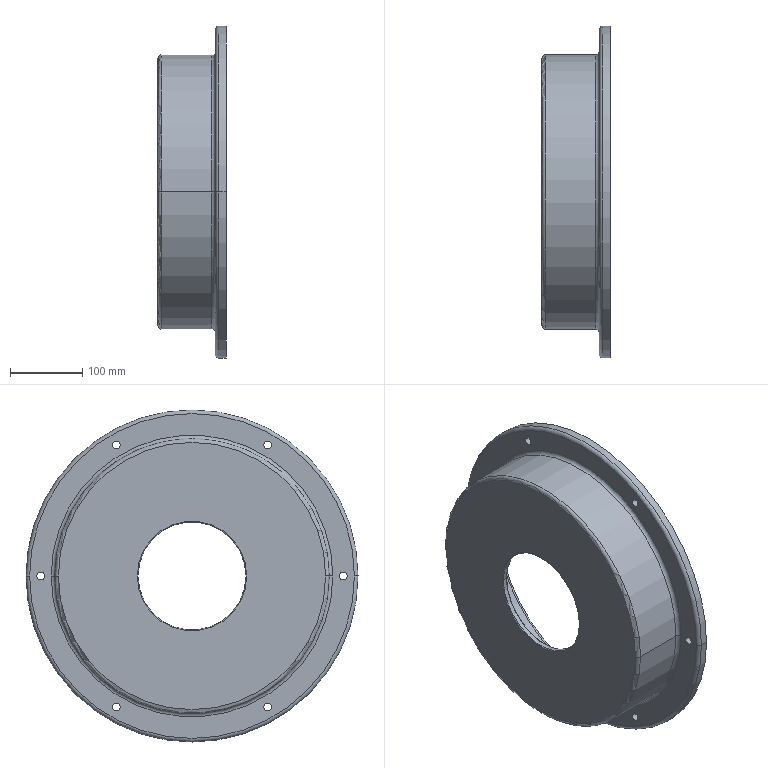Part | SolidWorks | features Cut 1, Revolution 1 | 1 solid | 43 faces | box 94.6 x 461 x 461 mm | volume 3440559 mm3 | cylinder 22 | torus 16 | plane 5 | commonest cylinder face diameters 11 x12 150 x2 225 x2 351 x2 381 x2 461 x2
STEP:
#1=CARTESIAN_POINT('',(298.52,204.5,0.));
#2=VERTEX_POINT('',#1);
#3=CARTESIAN_POINT('',(298.52,215.5,0.));
#4=VERTEX_POINT('',#3);
#5=CARTESIAN_POINT('',(298.52,210.,0.));
#6=DIRECTION('',(1.,0.,0.));
#7=DIRECTION('',(0.,1.,0.));
#8=AXIS2_PLACEMENT_3D('',#5,#6,#7);
#9=CIRCLE('',#8,5.5);
#10=EDGE_CURVE('',#2,#4,#9,.T.);
#11=ORIENTED_EDGE('',*,*,#10,.T.);
#12=CARTESIAN_POINT('',(283.52,215.5,0.));
#13=VERTEX_POINT('',#12);
#14=CARTESIAN_POINT('',(368.52,215.5,0.));
#15=DIRECTION('',(-1.,0.,0.));
#16=VECTOR('',#15,1000.);
#17=LINE('',#14,#16);
#18=EDGE_CURVE('',#4,#13,#17,.T.);
#19=ORIENTED_EDGE('',*,*,#18,.T.);
#20=CARTESIAN_POINT('',(283.52,204.5,0.));
#21=VERTEX_POINT('',#20);
#22=CARTESIAN_POINT('',(283.52,210.,0.));
#23=DIRECTION('',(-1.,0.,0.));
#24=DIRECTION('',(0.,-1.,0.));
#25=AXIS2_PLACEMENT_3D('',#22,#23,#24);
#26=CIRCLE('',#25,5.5);
#27=EDGE_CURVE('',#13,#21,#26,.T.);
#28=ORIENTED_EDGE('',*,*,#27,.T.);
#29=CARTESIAN_POINT('',(368.52,204.5,0.));
#30=DIRECTION('',(-1.,0.,0.));
#31=VECTOR('',#30,1000.);
#32=LINE('',#29,#31);
#33=EDGE_CURVE('',#2,#21,#32,.T.);
#34=ORIENTED_EDGE('',*,*,#33,.F.);
#35=EDGE_LOOP('',(#11,#19,#28,#34));
#36=FACE_OUTER_BOUND('',#35,.T.);
#37=CARTESIAN_POINT('',(368.52,210.,0.));
#38=DIRECTION('',(-1.,0.,0.));
#39=DIRECTION('',(0.,-1.,0.));
#40=AXIS2_PLACEMENT_3D('',#37,#38,#39);
#41=CYLINDRICAL_SURFACE('',#40,5.5);
#42=ADVANCED_FACE('',(#36),#41,.F.);
#43=CARTESIAN_POINT('',(298.52,99.5,-181.865));
#44=VERTEX_POINT('',#43);
#45=CARTESIAN_POINT('',(298.52,110.5,-181.865));
#46=VERTEX_POINT('',#45);
#47=CARTESIAN_POINT('',(298.52,105.,-181.865));
#48=DIRECTION('',(1.,0.,0.));
#49=DIRECTION('',(0.,1.,0.));
#50=AXIS2_PLACEMENT_3D('',#47,#48,#49);
#51=CIRCLE('',#50,5.5);
#52=EDGE_CURVE('',#44,#46,#51,.T.);
#53=ORIENTED_EDGE('',*,*,#52,.T.);
#54=CARTESIAN_POINT('',(283.52,110.5,-181.865));
#55=VERTEX_POINT('',#54);
#56=CARTESIAN_POINT('',(368.52,110.5,-181.865));
#57=DIRECTION('',(-1.,0.,0.));
#58=VECTOR('',#57,1000.);
#59=LINE('',#56,#58);
#60=EDGE_CURVE('',#46,#55,#59,.T.);
#61=ORIENTED_EDGE('',*,*,#60,.T.);
#62=CARTESIAN_POINT('',(283.52,99.5,-181.865));
#63=VERTEX_POINT('',#62);
#64=CARTESIAN_POINT('',(283.52,105.,-181.865));
#65=DIRECTION('',(-1.,0.,0.));
#66=DIRECTION('',(0.,-1.,0.));
#67=AXIS2_PLACEMENT_3D('',#64,#65,#66);
#68=CIRCLE('',#67,5.5);
#69=EDGE_CURVE('',#55,#63,#68,.T.);
#70=ORIENTED_EDGE('',*,*,#69,.T.);
#71=CARTESIAN_POINT('',(368.52,99.5,-181.865));
#72=DIRECTION('',(-1.,0.,0.));
#73=VECTOR('',#72,1000.);
#74=LINE('',#71,#73);
#75=EDGE_CURVE('',#44,#63,#74,.T.);
#76=ORIENTED_EDGE('',*,*,#75,.F.);
#77=EDGE_LOOP('',(#53,#61,#70,#76));
#78=FACE_OUTER_BOUND('',#77,.T.);
#79=CARTESIAN_POINT('',(368.52,105.,-181.865));
#80=DIRECTION('',(-1.,0.,0.));
#81=DIRECTION('',(0.,-1.,0.));
#82=AXIS2_PLACEMENT_3D('',#79,#80,#81);
#83=CYLINDRICAL_SURFACE('',#82,5.5);
#84=ADVANCED_FACE('',(#78),#83,.F.);
#85=CARTESIAN_POINT('',(298.52,-110.5,-181.865));
#86=VERTEX_POINT('',#85);
#87=CARTESIAN_POINT('',(298.52,-99.5,-181.865));
#88=VERTEX_POINT('',#87);
#89=CARTESIAN_POINT('',(298.52,-105.,-181.865));
#90=DIRECTION('',(1.,0.,0.));
#91=DIRECTION('',(0.,1.,0.));
#92=AXIS2_PLACEMENT_3D('',#89,#90,#91);
#93=CIRCLE('',#92,5.5);
#94=EDGE_CURVE('',#86,#88,#93,.T.);
#95=ORIENTED_EDGE('',*,*,#94,.T.);
#96=CARTESIAN_POINT('',(283.52,-99.5,-181.865));
#97=VERTEX_POINT('',#96);
#98=CARTESIAN_POINT('',(368.52,-99.5,-181.865));
#99=DIRECTION('',(-1.,0.,0.));
#100=VECTOR('',#99,1000.);
#101=LINE('',#98,#100);
#102=EDGE_CURVE('',#88,#97,#101,.T.);
#103=ORIENTED_EDGE('',*,*,#102,.T.);
#104=CARTESIAN_POINT('',(283.52,-110.5,-181.865));
#105=VERTEX_POINT('',#104);
#106=CARTESIAN_POINT('',(283.52,-105.,-181.865));
#107=DIRECTION('',(-1.,0.,0.));
#108=DIRECTION('',(0.,-1.,0.));
#109=AXIS2_PLACEMENT_3D('',#106,#107,#108);
#110=CIRCLE('',#109,5.5);
#111=EDGE_CURVE('',#97,#105,#110,.T.);
#112=ORIENTED_EDGE('',*,*,#111,.T.);
#113=CARTESIAN_POINT('',(368.52,-110.5,-181.865));
#114=DIRECTION('',(-1.,0.,0.));
#115=VECTOR('',#114,1000.);
#116=LINE('',#113,#115);
#117=EDGE_CURVE('',#86,#105,#116,.T.);
#118=ORIENTED_EDGE('',*,*,#117,.F.);
#119=EDGE_LOOP('',(#95,#103,#112,#118));
#120=FACE_OUTER_BOUND('',#119,.T.);
#121=CARTESIAN_POINT('',(368.52,-105.,-181.865));
#122=DIRECTION('',(-1.,0.,0.));
#123=DIRECTION('',(0.,-1.,0.));
#124=AXIS2_PLACEMENT_3D('',#121,#122,#123);
#125=CYLINDRICAL_SURFACE('',#124,5.5);
#126=ADVANCED_FACE('',(#120),#125,.F.);
#127=CARTESIAN_POINT('',(298.52,-215.5,0.));
#128=VERTEX_POINT('',#127);
#129=CARTESIAN_POINT('',(298.52,-204.5,0.));
#130=VERTEX_POINT('',#129);
#131=CARTESIAN_POINT('',(298.52,-210.,0.));
#132=DIRECTION('',(1.,0.,0.));
#133=DIRECTION('',(0.,1.,0.));
#134=AXIS2_PLACEMENT_3D('',#131,#132,#133);
#135=CIRCLE('',#134,5.5);
#136=EDGE_CURVE('',#128,#130,#135,.T.);
#137=ORIENTED_EDGE('',*,*,#136,.T.);
#138=CARTESIAN_POINT('',(283.52,-204.5,0.));
#139=VERTEX_POINT('',#138);
#140=CARTESIAN_POINT('',(368.52,-204.5,0.));
#141=DIRECTION('',(-1.,0.,0.));
#142=VECTOR('',#141,1000.);
#143=LINE('',#140,#142);
#144=EDGE_CURVE('',#130,#139,#143,.T.);
#145=ORIENTED_EDGE('',*,*,#144,.T.);
#146=CARTESIAN_POINT('',(283.52,-215.5,0.));
#147=VERTEX_POINT('',#146);
#148=CARTESIAN_POINT('',(283.52,-210.,0.));
#149=DIRECTION('',(-1.,0.,0.));
#150=DIRECTION('',(0.,-1.,0.));
#151=AXIS2_PLACEMENT_3D('',#148,#149,#150);
#152=CIRCLE('',#151,5.5);
#153=EDGE_CURVE('',#139,#147,#152,.T.);
#154=ORIENTED_EDGE('',*,*,#153,.T.);
#155=CARTESIAN_POINT('',(368.52,-215.5,0.));
#156=DIRECTION('',(-1.,0.,0.));
#157=VECTOR('',#156,1000.);
#158=LINE('',#155,#157);
#159=EDGE_CURVE('',#128,#147,#158,.T.);
#160=ORIENTED_EDGE('',*,*,#159,.F.);
#161=EDGE_LOOP('',(#137,#145,#154,#160));
#162=FACE_OUTER_BOUND('',#161,.T.);
#163=CARTESIAN_POINT('',(368.52,-210.,0.));
#164=DIRECTION('',(-1.,0.,0.));
#165=DIRECTION('',(0.,-1.,0.));
#166=AXIS2_PLACEMENT_3D('',#163,#164,#165);
#167=CYLINDRICAL_SURFACE('',#166,5.5);
#168=ADVANCED_FACE('',(#162),#167,.F.);
#169=CARTESIAN_POINT('',(298.52,-110.5,181.865));
#170=VERTEX_POINT('',#169);
#171=CARTESIAN_POINT('',(298.52,-99.5,181.865));
#172=VERTEX_POINT('',#171);
#173=CARTESIAN_POINT('',(298.52,-105.,181.865));
#174=DIRECTION('',(1.,0.,0.));
#175=DIRECTION('',(0.,1.,0.));
#176=AXIS2_PLACEMENT_3D('',#173,#174,#175);
#177=CIRCLE('',#176,5.5);
#178=EDGE_CURVE('',#170,#172,#177,.T.);
#179=ORIENTED_EDGE('',*,*,#178,.T.);
#180=CARTESIAN_POINT('',(283.52,-99.5,181.865));
#181=VERTEX_POINT('',#180);
#182=CARTESIAN_POINT('',(368.52,-99.5,181.865));
#183=DIRECTION('',(-1.,0.,0.));
#184=VECTOR('',#183,1000.);
#185=LINE('',#182,#184);
#186=EDGE_CURVE('',#172,#181,#185,.T.);
#187=ORIENTED_EDGE('',*,*,#186,.T.);
#188=CARTESIAN_POINT('',(283.52,-110.5,181.865));
#189=VERTEX_POINT('',#188);
#190=CARTESIAN_POINT('',(283.52,-105.,181.865));
#191=DIRECTION('',(-1.,0.,0.));
#192=DIRECTION('',(0.,-1.,0.));
#193=AXIS2_PLACEMENT_3D('',#190,#191,#192);
#194=CIRCLE('',#193,5.5);
#195=EDGE_CURVE('',#181,#189,#194,.T.);
#196=ORIENTED_EDGE('',*,*,#195,.T.);
#197=CARTESIAN_POINT('',(368.52,-110.5,181.865));
#198=DIRECTION('',(-1.,0.,0.));
#199=VECTOR('',#198,1000.);
#200=LINE('',#197,#199);
#201=EDGE_CURVE('',#170,#189,#200,.T.);
#202=ORIENTED_EDGE('',*,*,#201,.F.);
#203=EDGE_LOOP('',(#179,#187,#196,#202));
#204=FACE_OUTER_BOUND('',#203,.T.);
#205=CARTESIAN_POINT('',(368.52,-105.,181.865));
#206=DIRECTION('',(-1.,0.,0.));
#207=DIRECTION('',(0.,-1.,0.));
#208=AXIS2_PLACEMENT_3D('',#205,#206,#207);
#209=CYLINDRICAL_SURFACE('',#208,5.5);
#210=ADVANCED_FACE('',(#204),#209,.F.);
#211=CARTESIAN_POINT('',(298.52,99.5,181.865));
#212=VERTEX_POINT('',#211);
#213=CARTESIAN_POINT('',(298.52,110.5,181.865));
#214=VERTEX_POINT('',#213);
#215=CARTESIAN_POINT('',(298.52,105.,181.865));
#216=DIRECTION('',(1.,0.,0.));
#217=DIRECTION('',(0.,1.,0.));
#218=AXIS2_PLACEMENT_3D('',#215,#216,#217);
#219=CIRCLE('',#218,5.5);
#220=EDGE_CURVE('',#212,#214,#219,.T.);
#221=ORIENTED_EDGE('',*,*,#220,.T.);
#222=CARTESIAN_POINT('',(283.52,110.5,181.865));
#223=VERTEX_POINT('',#222);
#224=CARTESIAN_POINT('',(368.52,110.5,181.865));
#225=DIRECTION('',(-1.,0.,0.));
#226=VECTOR('',#225,1000.);
#227=LINE('',#224,#226);
#228=EDGE_CURVE('',#214,#223,#227,.T.);
#229=ORIENTED_EDGE('',*,*,#228,.T.);
#230=CARTESIAN_POINT('',(283.52,99.5,181.865));
#231=VERTEX_POINT('',#230);
#232=CARTESIAN_POINT('',(283.52,105.,181.865));
#233=DIRECTION('',(-1.,0.,0.));
#234=DIRECTION('',(0.,-1.,0.));
#235=AXIS2_PLACEMENT_3D('',#232,#233,#234);
#236=CIRCLE('',#235,5.5);
#237=EDGE_CURVE('',#223,#231,#236,.T.);
#238=ORIENTED_EDGE('',*,*,#237,.T.);
#239=CARTESIAN_POINT('',(368.52,99.5,181.865));
#240=DIRECTION('',(-1.,0.,0.));
#241=VECTOR('',#240,1000.);
#242=LINE('',#239,#241);
#243=EDGE_CURVE('',#212,#231,#242,.T.);
#244=ORIENTED_EDGE('',*,*,#243,.F.);
#245=EDGE_LOOP('',(#221,#229,#238,#244));
#246=FACE_OUTER_BOUND('',#245,.T.);
#247=CARTESIAN_POINT('',(368.52,105.,181.865));
#248=DIRECTION('',(-1.,0.,0.));
#249=DIRECTION('',(0.,-1.,0.));
#250=AXIS2_PLACEMENT_3D('',#247,#248,#249);
#251=CYLINDRICAL_SURFACE('',#250,5.5);
#252=ADVANCED_FACE('',(#246),#251,.F.);
#253=CARTESIAN_POINT('',(212.92,-112.5,0.));
#254=VERTEX_POINT('',#253);
#255=CARTESIAN_POINT('',(212.92,112.5,0.));
#256=VERTEX_POINT('',#255);
#257=CARTESIAN_POINT('',(212.92,0.,0.));
#258=DIRECTION('',(1.,0.,0.));
#259=DIRECTION('',(0.,1.,0.));
#260=AXIS2_PLACEMENT_3D('',#257,#258,#259);
#261=CIRCLE('',#260,112.5);
#262=EDGE_CURVE('',#254,#256,#261,.T.);
#263=ORIENTED_EDGE('',*,*,#262,.F.);
#264=CARTESIAN_POINT('',(218.92,-112.5,0.));
#265=VERTEX_POINT('',#264);
#266=CARTESIAN_POINT('',(373.52,-112.5,0.));
#267=DIRECTION('',(1.,0.,0.));
#268=VECTOR('',#267,1000.);
#269=LINE('',#266,#268);
#270=EDGE_CURVE('',#254,#265,#269,.T.);
#271=ORIENTED_EDGE('',*,*,#270,.T.);
#272=CARTESIAN_POINT('',(218.92,112.5,0.));
#273=VERTEX_POINT('',#272);
#274=CARTESIAN_POINT('',(218.92,0.,0.));
#275=DIRECTION('',(1.,0.,0.));
#276=DIRECTION('',(0.,1.,0.));
#277=AXIS2_PLACEMENT_3D('',#274,#275,#276);
#278=CIRCLE('',#277,112.5);
#279=EDGE_CURVE('',#265,#273,#278,.T.);
#280=ORIENTED_EDGE('',*,*,#279,.T.);
#281=CARTESIAN_POINT('',(373.52,112.5,0.));
#282=DIRECTION('',(1.,0.,0.));
#283=VECTOR('',#282,1000.);
#284=LINE('',#281,#283);
#285=EDGE_CURVE('',#256,#273,#284,.T.);
#286=ORIENTED_EDGE('',*,*,#285,.F.);
#287=EDGE_LOOP('',(#263,#271,#280,#286));
#288=FACE_OUTER_BOUND('',#287,.T.);
#289=CARTESIAN_POINT('',(373.52,0.,0.));
#290=DIRECTION('',(1.,0.,0.));
#291=DIRECTION('',(0.,1.,0.));
#292=AXIS2_PLACEMENT_3D('',#289,#290,#291);
#293=CYLINDRICAL_SURFACE('',#292,112.5);
#294=ADVANCED_FACE('',(#288),#293,.F.);
#295=CARTESIAN_POINT('',(211.92,-111.5,0.));
#296=VERTEX_POINT('',#295);
#297=CARTESIAN_POINT('',(211.92,111.5,0.));
#298=VERTEX_POINT('',#297);
#299=CARTESIAN_POINT('',(211.92,0.,0.));
#300=DIRECTION('',(1.,0.,0.));
#301=DIRECTION('',(0.,1.,0.));
#302=AXIS2_PLACEMENT_3D('',#299,#300,#301);
#303=CIRCLE('',#302,111.5);
#304=EDGE_CURVE('',#296,#298,#303,.T.);
#305=ORIENTED_EDGE('',*,*,#304,.F.);
#306=CARTESIAN_POINT('',(212.92,-111.5,0.));
#307=DIRECTION('',(0.,0.,1.));
#308=DIRECTION('',(0.,-1.,0.));
#309=AXIS2_PLACEMENT_3D('',#306,#307,#308);
#310=CIRCLE('',#309,1.);
#311=EDGE_CURVE('',#296,#254,#310,.T.);
#312=ORIENTED_EDGE('',*,*,#311,.T.);
#313=ORIENTED_EDGE('',*,*,#262,.T.);
#314=CARTESIAN_POINT('',(212.92,111.5,0.));
#315=DIRECTION('',(0.,0.,-1.));
#316=DIRECTION('',(-1.,0.,0.));
#317=AXIS2_PLACEMENT_3D('',#314,#315,#316);
#318=CIRCLE('',#317,1.);
#319=EDGE_CURVE('',#298,#256,#318,.T.);
#320=ORIENTED_EDGE('',*,*,#319,.F.);
#321=EDGE_LOOP('',(#305,#312,#313,#320));
#322=FACE_OUTER_BOUND('',#321,.T.);
#323=CARTESIAN_POINT('',(212.92,0.,0.));
#324=DIRECTION('',(1.,0.,0.));
#325=DIRECTION('',(0.,1.,0.));
#326=AXIS2_PLACEMENT_3D('',#323,#324,#325);
#327=TOROIDAL_SURFACE('',#326,111.5,1.);
#328=ADVANCED_FACE('',(#322),#327,.F.);
#329=CARTESIAN_POINT('',(211.92,76.,0.));
#330=VERTEX_POINT('',#329);
#331=CARTESIAN_POINT('',(211.92,-76.,0.));
#332=VERTEX_POINT('',#331);
#333=CARTESIAN_POINT('',(211.92,0.,0.));
#334=DIRECTION('',(1.,0.,0.));
#335=DIRECTION('',(0.,1.,0.));
#336=AXIS2_PLACEMENT_3D('',#333,#334,#335);
#337=CIRCLE('',#336,76.);
#338=EDGE_CURVE('',#330,#332,#337,.T.);
#339=ORIENTED_EDGE('',*,*,#338,.T.);
#340=CARTESIAN_POINT('',(210.92,-75.,0.));
#341=VERTEX_POINT('',#340);
#342=CARTESIAN_POINT('',(210.92,-76.,0.));
#343=DIRECTION('',(0.,0.,1.));
#344=DIRECTION('',(0.,-1.,0.));
#345=AXIS2_PLACEMENT_3D('',#342,#343,#344);
#346=CIRCLE('',#345,1.);
#347=EDGE_CURVE('',#332,#341,#346,.T.);
#348=ORIENTED_EDGE('',*,*,#347,.T.);
#349=CARTESIAN_POINT('',(210.92,75.,0.));
#350=VERTEX_POINT('',#349);
#351=CARTESIAN_POINT('',(210.92,0.,0.));
#352=DIRECTION('',(1.,0.,0.));
#353=DIRECTION('',(0.,1.,0.));
#354=AXIS2_PLACEMENT_3D('',#351,#352,#353);
#355=CIRCLE('',#354,75.);
#356=EDGE_CURVE('',#350,#341,#355,.T.);
#357=ORIENTED_EDGE('',*,*,#356,.F.);
#358=CARTESIAN_POINT('',(210.92,76.,0.));
#359=DIRECTION('',(0.,0.,-1.));
#360=DIRECTION('',(-1.,0.,0.));
#361=AXIS2_PLACEMENT_3D('',#358,#359,#360);
#362=CIRCLE('',#361,1.);
#363=EDGE_CURVE('',#330,#350,#362,.T.);
#364=ORIENTED_EDGE('',*,*,#363,.F.);
#365=EDGE_LOOP('',(#339,#348,#357,#364));
#366=FACE_OUTER_BOUND('',#365,.T.);
#367=CARTESIAN_POINT('',(210.92,0.,0.));
#368=DIRECTION('',(1.,0.,0.));
#369=DIRECTION('',(0.,1.,0.));
#370=AXIS2_PLACEMENT_3D('',#367,#368,#369);
#371=TOROIDAL_SURFACE('',#370,76.,1.);
#372=ADVANCED_FACE('',(#366),#371,.T.);
#373=CARTESIAN_POINT('',(204.92,-75.,0.));
#374=VERTEX_POINT('',#373);
#375=CARTESIAN_POINT('',(204.92,75.,0.));
#376=VERTEX_POINT('',#375);
#377=CARTESIAN_POINT('',(204.92,0.,0.));
#378=DIRECTION('',(1.,0.,0.));
#379=DIRECTION('',(0.,1.,0.));
#380=AXIS2_PLACEMENT_3D('',#377,#378,#379);
#381=CIRCLE('',#380,75.);
#382=EDGE_CURVE('',#374,#376,#381,.T.);
#383=ORIENTED_EDGE('',*,*,#382,.F.);
#384=CARTESIAN_POINT('',(373.52,-75.,0.));
#385=DIRECTION('',(1.,0.,0.));
#386=VECTOR('',#385,1000.);
#387=LINE('',#384,#386);
#388=EDGE_CURVE('',#374,#341,#387,.T.);
#389=ORIENTED_EDGE('',*,*,#388,.T.);
#390=CARTESIAN_POINT('',(210.92,0.,0.));
#391=DIRECTION('',(1.,0.,0.));
#392=DIRECTION('',(0.,1.,0.));
#393=AXIS2_PLACEMENT_3D('',#390,#391,#392);
#394=CIRCLE('',#393,75.);
#395=EDGE_CURVE('',#341,#350,#394,.T.);
#396=ORIENTED_EDGE('',*,*,#395,.T.);
#397=CARTESIAN_POINT('',(373.52,75.,0.));
#398=DIRECTION('',(1.,0.,0.));
#399=VECTOR('',#398,1000.);
#400=LINE('',#397,#399);
#401=EDGE_CURVE('',#376,#350,#400,.T.);
#402=ORIENTED_EDGE('',*,*,#401,.F.);
#403=EDGE_LOOP('',(#383,#389,#396,#402));
#404=FACE_OUTER_BOUND('',#403,.T.);
#405=CARTESIAN_POINT('',(373.52,0.,0.));
#406=DIRECTION('',(1.,0.,0.));
#407=DIRECTION('',(0.,1.,0.));
#408=AXIS2_PLACEMENT_3D('',#405,#406,#407);
#409=CYLINDRICAL_SURFACE('',#408,75.);
#410=ADVANCED_FACE('',(#404),#409,.F.);
#411=CARTESIAN_POINT('',(204.92,0.,0.));
#412=DIRECTION('',(1.,0.,0.));
#413=DIRECTION('',(0.,1.,0.));
#414=AXIS2_PLACEMENT_3D('',#411,#412,#413);
#415=CIRCLE('',#414,75.);
#416=EDGE_CURVE('',#376,#374,#415,.T.);
#417=ORIENTED_EDGE('',*,*,#416,.T.);
#418=CARTESIAN_POINT('',(203.92,-76.,0.));
#419=VERTEX_POINT('',#418);
#420=CARTESIAN_POINT('',(204.92,-76.,0.));
#421=DIRECTION('',(0.,0.,1.));
#422=DIRECTION('',(0.,-1.,0.));
#423=AXIS2_PLACEMENT_3D('',#420,#421,#422);
#424=CIRCLE('',#423,1.);
#425=EDGE_CURVE('',#374,#419,#424,.T.);
#426=ORIENTED_EDGE('',*,*,#425,.T.);
#427=CARTESIAN_POINT('',(203.92,76.,0.));
#428=VERTEX_POINT('',#427);
#429=CARTESIAN_POINT('',(203.92,0.,0.));
#430=DIRECTION('',(1.,0.,0.));
#431=DIRECTION('',(0.,1.,0.));
#432=AXIS2_PLACEMENT_3D('',#429,#430,#431);
#433=CIRCLE('',#432,76.);
#434=EDGE_CURVE('',#428,#419,#433,.T.);
#435=ORIENTED_EDGE('',*,*,#434,.F.);
#436=CARTESIAN_POINT('',(204.92,76.,0.));
#437=DIRECTION('',(0.,0.,-1.));
#438=DIRECTION('',(-1.,0.,0.));
#439=AXIS2_PLACEMENT_3D('',#436,#437,#438);
#440=CIRCLE('',#439,1.);
#441=EDGE_CURVE('',#376,#428,#440,.T.);
#442=ORIENTED_EDGE('',*,*,#441,.F.);
#443=EDGE_LOOP('',(#417,#426,#435,#442));
#444=FACE_OUTER_BOUND('',#443,.T.);
#445=CARTESIAN_POINT('',(204.92,0.,0.));
#446=DIRECTION('',(1.,0.,0.));
#447=DIRECTION('',(0.,1.,0.));
#448=AXIS2_PLACEMENT_3D('',#445,#446,#447);
#449=TOROIDAL_SURFACE('',#448,76.,1.);
#450=ADVANCED_FACE('',(#444),#449,.T.);
#451=CARTESIAN_POINT('',(203.92,185.5,0.));
#452=VERTEX_POINT('',#451);
#453=CARTESIAN_POINT('',(203.92,-185.5,0.));
#454=VERTEX_POINT('',#453);
#455=CARTESIAN_POINT('',(203.92,0.,0.));
#456=DIRECTION('',(1.,0.,0.));
#457=DIRECTION('',(0.,1.,0.));
#458=AXIS2_PLACEMENT_3D('',#455,#456,#457);
#459=CIRCLE('',#458,185.5);
#460=EDGE_CURVE('',#452,#454,#459,.T.);
#461=ORIENTED_EDGE('',*,*,#460,.T.);
#462=CARTESIAN_POINT('',(208.92,-190.5,0.));
#463=VERTEX_POINT('',#462);
#464=CARTESIAN_POINT('',(208.92,-185.5,0.));
#465=DIRECTION('',(0.,0.,1.));
#466=DIRECTION('',(0.,-1.,0.));
#467=AXIS2_PLACEMENT_3D('',#464,#465,#466);
#468=CIRCLE('',#467,5.);
#469=EDGE_CURVE('',#454,#463,#468,.T.);
#470=ORIENTED_EDGE('',*,*,#469,.T.);
#471=CARTESIAN_POINT('',(208.92,190.5,0.));
#472=VERTEX_POINT('',#471);
#473=CARTESIAN_POINT('',(208.92,0.,0.));
#474=DIRECTION('',(1.,0.,0.));
#475=DIRECTION('',(0.,1.,0.));
#476=AXIS2_PLACEMENT_3D('',#473,#474,#475);
#477=CIRCLE('',#476,190.5);
#478=EDGE_CURVE('',#472,#463,#477,.T.);
#479=ORIENTED_EDGE('',*,*,#478,.F.);
#480=CARTESIAN_POINT('',(208.92,185.5,0.));
#481=DIRECTION('',(0.,0.,-1.));
#482=DIRECTION('',(-1.,0.,0.));
#483=AXIS2_PLACEMENT_3D('',#480,#481,#482);
#484=CIRCLE('',#483,5.);
#485=EDGE_CURVE('',#452,#472,#484,.T.);
#486=ORIENTED_EDGE('',*,*,#485,.F.);
#487=EDGE_LOOP('',(#461,#470,#479,#486));
#488=FACE_OUTER_BOUND('',#487,.T.);
#489=CARTESIAN_POINT('',(208.92,0.,0.));
#490=DIRECTION('',(1.,0.,0.));
#491=DIRECTION('',(0.,1.,0.));
#492=AXIS2_PLACEMENT_3D('',#489,#490,#491);
#493=TOROIDAL_SURFACE('',#492,185.5,5.);
#494=ADVANCED_FACE('',(#488),#493,.T.);
#495=ORIENTED_EDGE('',*,*,#478,.T.);
#496=CARTESIAN_POINT('',(278.52,-190.5,0.));
#497=VERTEX_POINT('',#496);
#498=CARTESIAN_POINT('',(373.52,-190.5,0.));
#499=DIRECTION('',(1.,0.,0.));
#500=VECTOR('',#499,1000.);
#501=LINE('',#498,#500);
#502=EDGE_CURVE('',#463,#497,#501,.T.);
#503=ORIENTED_EDGE('',*,*,#502,.T.);
#504=CARTESIAN_POINT('',(278.52,190.5,0.));
#505=VERTEX_POINT('',#504);
#506=CARTESIAN_POINT('',(278.52,0.,0.));
#507=DIRECTION('',(1.,0.,0.));
#508=DIRECTION('',(0.,1.,0.));
#509=AXIS2_PLACEMENT_3D('',#506,#507,#508);
#510=CIRCLE('',#509,190.5);
#511=EDGE_CURVE('',#505,#497,#510,.T.);
#512=ORIENTED_EDGE('',*,*,#511,.F.);
#513=CARTESIAN_POINT('',(373.52,190.5,0.));
#514=DIRECTION('',(1.,0.,0.));
#515=VECTOR('',#514,1000.);
#516=LINE('',#513,#515);
#517=EDGE_CURVE('',#472,#505,#516,.T.);
#518=ORIENTED_EDGE('',*,*,#517,.F.);
#519=EDGE_LOOP('',(#495,#503,#512,#518));
#520=FACE_OUTER_BOUND('',#519,.T.);
#521=CARTESIAN_POINT('',(373.52,0.,0.));
#522=DIRECTION('',(1.,0.,0.));
#523=DIRECTION('',(0.,1.,0.));
#524=AXIS2_PLACEMENT_3D('',#521,#522,#523);
#525=CYLINDRICAL_SURFACE('',#524,190.5);
#526=ADVANCED_FACE('',(#520),#525,.T.);
#527=CARTESIAN_POINT('',(283.52,-195.5,0.));
#528=VERTEX_POINT('',#527);
#529=CARTESIAN_POINT('',(283.52,195.5,0.));
#530=VERTEX_POINT('',#529);
#531=CARTESIAN_POINT('',(283.52,0.,0.));
#532=DIRECTION('',(1.,0.,0.));
#533=DIRECTION('',(0.,1.,0.));
#534=AXIS2_PLACEMENT_3D('',#531,#532,#533);
#535=CIRCLE('',#534,195.5);
#536=EDGE_CURVE('',#528,#530,#535,.T.);
#537=ORIENTED_EDGE('',*,*,#536,.F.);
#538=CARTESIAN_POINT('',(278.52,-195.5,0.));
#539=DIRECTION('',(0.,0.,1.));
#540=DIRECTION('',(0.,-1.,0.));
#541=AXIS2_PLACEMENT_3D('',#538,#539,#540);
#542=CIRCLE('',#541,5.);
#543=EDGE_CURVE('',#528,#497,#542,.T.);
#544=ORIENTED_EDGE('',*,*,#543,.T.);
#545=CARTESIAN_POINT('',(278.52,0.,0.));
#546=DIRECTION('',(1.,0.,0.));
#547=DIRECTION('',(0.,1.,0.));
#548=AXIS2_PLACEMENT_3D('',#545,#546,#547);
#549=CIRCLE('',#548,190.5);
#550=EDGE_CURVE('',#497,#505,#549,.T.);
#551=ORIENTED_EDGE('',*,*,#550,.T.);
#552=CARTESIAN_POINT('',(278.52,195.5,0.));
#553=DIRECTION('',(0.,0.,-1.));
#554=DIRECTION('',(-1.,0.,0.));
#555=AXIS2_PLACEMENT_3D('',#552,#553,#554);
#556=CIRCLE('',#555,5.);
#557=EDGE_CURVE('',#530,#505,#556,.T.);
#558=ORIENTED_EDGE('',*,*,#557,.F.);
#559=EDGE_LOOP('',(#537,#544,#551,#558));
#560=FACE_OUTER_BOUND('',#559,.T.);
#561=CARTESIAN_POINT('',(278.52,0.,0.));
#562=DIRECTION('',(1.,0.,0.));
#563=DIRECTION('',(0.,1.,0.));
#564=AXIS2_PLACEMENT_3D('',#561,#562,#563);
#565=TOROIDAL_SURFACE('',#564,195.5,5.);
#566=ADVANCED_FACE('',(#560),#565,.F.);
#567=CARTESIAN_POINT('',(283.52,225.5,0.));
#568=VERTEX_POINT('',#567);
#569=CARTESIAN_POINT('',(283.52,-225.5,0.));
#570=VERTEX_POINT('',#569);
#571=CARTESIAN_POINT('',(283.52,0.,0.));
#572=DIRECTION('',(1.,0.,0.));
#573=DIRECTION('',(0.,1.,0.));
#574=AXIS2_PLACEMENT_3D('',#571,#572,#573);
#575=CIRCLE('',#574,225.5);
#576=EDGE_CURVE('',#568,#570,#575,.T.);
#577=ORIENTED_EDGE('',*,*,#576,.T.);
#578=CARTESIAN_POINT('',(288.52,-230.5,0.));
#579=VERTEX_POINT('',#578);
#580=CARTESIAN_POINT('',(288.52,-225.5,0.));
#581=DIRECTION('',(0.,0.,1.));
#582=DIRECTION('',(0.,-1.,0.));
#583=AXIS2_PLACEMENT_3D('',#580,#581,#582);
#584=CIRCLE('',#583,5.);
#585=EDGE_CURVE('',#570,#579,#584,.T.);
#586=ORIENTED_EDGE('',*,*,#585,.T.);
#587=CARTESIAN_POINT('',(288.52,230.5,0.));
#588=VERTEX_POINT('',#587);
#589=CARTESIAN_POINT('',(288.52,0.,0.));
#590=DIRECTION('',(1.,0.,0.));
#591=DIRECTION('',(0.,1.,0.));
#592=AXIS2_PLACEMENT_3D('',#589,#590,#591);
#593=CIRCLE('',#592,230.5);
#594=EDGE_CURVE('',#588,#579,#593,.T.);
#595=ORIENTED_EDGE('',*,*,#594,.F.);
#596=CARTESIAN_POINT('',(288.52,225.5,0.));
#597=DIRECTION('',(0.,0.,-1.));
#598=DIRECTION('',(-1.,0.,0.));
#599=AXIS2_PLACEMENT_3D('',#596,#597,#598);
#600=CIRCLE('',#599,5.);
#601=EDGE_CURVE('',#568,#588,#600,.T.);
#602=ORIENTED_EDGE('',*,*,#601,.F.);
#603=EDGE_LOOP('',(#577,#586,#595,#602));
#604=FACE_OUTER_BOUND('',#603,.T.);
#605=CARTESIAN_POINT('',(288.52,0.,0.));
#606=DIRECTION('',(1.,0.,0.));
#607=DIRECTION('',(0.,1.,0.));
#608=AXIS2_PLACEMENT_3D('',#605,#606,#607);
#609=TOROIDAL_SURFACE('',#608,225.5,5.);
#610=ADVANCED_FACE('',(#604),#609,.T.);
#611=ORIENTED_EDGE('',*,*,#594,.T.);
#612=CARTESIAN_POINT('',(298.52,-230.5,0.));
#613=VERTEX_POINT('',#612);
#614=CARTESIAN_POINT('',(373.52,-230.5,0.));
#615=DIRECTION('',(1.,0.,0.));
#616=VECTOR('',#615,1000.);
#617=LINE('',#614,#616);
#618=EDGE_CURVE('',#579,#613,#617,.T.);
#619=ORIENTED_EDGE('',*,*,#618,.T.);
#620=CARTESIAN_POINT('',(298.52,230.5,0.));
#621=VERTEX_POINT('',#620);
#622=CARTESIAN_POINT('',(298.52,0.,0.));
#623=DIRECTION('',(1.,0.,0.));
#624=DIRECTION('',(0.,1.,0.));
#625=AXIS2_PLACEMENT_3D('',#622,#623,#624);
#626=CIRCLE('',#625,230.5);
#627=EDGE_CURVE('',#621,#613,#626,.T.);
#628=ORIENTED_EDGE('',*,*,#627,.F.);
#629=CARTESIAN_POINT('',(373.52,230.5,0.));
#630=DIRECTION('',(1.,0.,0.));
#631=VECTOR('',#630,1000.);
#632=LINE('',#629,#631);
#633=EDGE_CURVE('',#588,#621,#632,.T.);
#634=ORIENTED_EDGE('',*,*,#633,.F.);
#635=EDGE_LOOP('',(#611,#619,#628,#634));
#636=FACE_OUTER_BOUND('',#635,.T.);
#637=CARTESIAN_POINT('',(373.52,0.,0.));
#638=DIRECTION('',(1.,0.,0.));
#639=DIRECTION('',(0.,1.,0.));
#640=AXIS2_PLACEMENT_3D('',#637,#638,#639);
#641=CYLINDRICAL_SURFACE('',#640,230.5);
#642=ADVANCED_FACE('',(#636),#641,.T.);
#643=CARTESIAN_POINT('',(298.52,180.5,0.));
#644=VERTEX_POINT('',#643);
#645=CARTESIAN_POINT('',(298.52,-180.5,0.));
#646=VERTEX_POINT('',#645);
#647=CARTESIAN_POINT('',(298.52,0.,0.));
#648=DIRECTION('',(1.,0.,0.));
#649=DIRECTION('',(0.,1.,0.));
#650=AXIS2_PLACEMENT_3D('',#647,#648,#649);
#651=CIRCLE('',#650,180.5);
#652=EDGE_CURVE('',#644,#646,#651,.T.);
#653=ORIENTED_EDGE('',*,*,#652,.T.);
#654=CARTESIAN_POINT('',(293.52,-175.5,0.));
#655=VERTEX_POINT('',#654);
#656=CARTESIAN_POINT('',(293.52,-180.5,0.));
#657=DIRECTION('',(0.,0.,1.));
#658=DIRECTION('',(0.,-1.,0.));
#659=AXIS2_PLACEMENT_3D('',#656,#657,#658);
#660=CIRCLE('',#659,5.);
#661=EDGE_CURVE('',#646,#655,#660,.T.);
#662=ORIENTED_EDGE('',*,*,#661,.T.);
#663=CARTESIAN_POINT('',(293.52,175.5,0.));
#664=VERTEX_POINT('',#663);
#665=CARTESIAN_POINT('',(293.52,0.,0.));
#666=DIRECTION('',(1.,0.,0.));
#667=DIRECTION('',(0.,1.,0.));
#668=AXIS2_PLACEMENT_3D('',#665,#666,#667);
#669=CIRCLE('',#668,175.5);
#670=EDGE_CURVE('',#664,#655,#669,.T.);
#671=ORIENTED_EDGE('',*,*,#670,.F.);
#672=CARTESIAN_POINT('',(293.52,180.5,0.));
#673=DIRECTION('',(0.,0.,-1.));
#674=DIRECTION('',(-1.,0.,0.));
#675=AXIS2_PLACEMENT_3D('',#672,#673,#674);
#676=CIRCLE('',#675,5.);
#677=EDGE_CURVE('',#644,#664,#676,.T.);
#678=ORIENTED_EDGE('',*,*,#677,.F.);
#679=EDGE_LOOP('',(#653,#662,#671,#678));
#680=FACE_OUTER_BOUND('',#679,.T.);
#681=CARTESIAN_POINT('',(293.52,0.,0.));
#682=DIRECTION('',(1.,0.,0.));
#683=DIRECTION('',(0.,1.,0.));
#684=AXIS2_PLACEMENT_3D('',#681,#682,#683);
#685=TOROIDAL_SURFACE('',#684,180.5,5.);
#686=ADVANCED_FACE('',(#680),#685,.T.);
#687=CARTESIAN_POINT('',(223.92,-175.5,0.));
#688=VERTEX_POINT('',#687);
#689=CARTESIAN_POINT('',(223.92,175.5,0.));
#690=VERTEX_POINT('',#689);
#691=CARTESIAN_POINT('',(223.92,0.,0.));
#692=DIRECTION('',(1.,0.,0.));
#693=DIRECTION('',(0.,1.,0.));
#694=AXIS2_PLACEMENT_3D('',#691,#692,#693);
#695=CIRCLE('',#694,175.5);
#696=EDGE_CURVE('',#688,#690,#695,.T.);
#697=ORIENTED_EDGE('',*,*,#696,.F.);
#698=CARTESIAN_POINT('',(373.52,-175.5,0.));
#699=DIRECTION('',(1.,0.,0.));
#700=VECTOR('',#699,1000.);
#701=LINE('',#698,#700);
#702=EDGE_CURVE('',#688,#655,#701,.T.);
#703=ORIENTED_EDGE('',*,*,#702,.T.);
#704=CARTESIAN_POINT('',(293.52,0.,0.));
#705=DIRECTION('',(1.,0.,0.));
#706=DIRECTION('',(0.,1.,0.));
#707=AXIS2_PLACEMENT_3D('',#704,#705,#706);
#708=CIRCLE('',#707,175.5);
#709=EDGE_CURVE('',#655,#664,#708,.T.);
#710=ORIENTED_EDGE('',*,*,#709,.T.);
#711=CARTESIAN_POINT('',(373.52,175.5,0.));
#712=DIRECTION('',(1.,0.,0.));
#713=VECTOR('',#712,1000.);
#714=LINE('',#711,#713);
#715=EDGE_CURVE('',#690,#664,#714,.T.);
#716=ORIENTED_EDGE('',*,*,#715,.F.);
#717=EDGE_LOOP('',(#697,#703,#710,#716));
#718=FACE_OUTER_BOUND('',#717,.T.);
#719=CARTESIAN_POINT('',(373.52,0.,0.));
#720=DIRECTION('',(1.,0.,0.));
#721=DIRECTION('',(0.,1.,0.));
#722=AXIS2_PLACEMENT_3D('',#719,#720,#721);
#723=CYLINDRICAL_SURFACE('',#722,175.5);
#724=ADVANCED_FACE('',(#718),#723,.F.);
#725=CARTESIAN_POINT('',(218.92,-170.5,0.));
#726=VERTEX_POINT('',#725);
#727=CARTESIAN_POINT('',(218.92,170.5,0.));
#728=VERTEX_POINT('',#727);
#729=CARTESIAN_POINT('',(218.92,0.,0.));
#730=DIRECTION('',(1.,0.,0.));
#731=DIRECTION('',(0.,1.,0.));
#732=AXIS2_PLACEMENT_3D('',#729,#730,#731);
#733=CIRCLE('',#732,170.5);
#734=EDGE_CURVE('',#726,#728,#733,.T.);
#735=ORIENTED_EDGE('',*,*,#734,.F.);
#736=CARTESIAN_POINT('',(223.92,-170.5,0.));
#737=DIRECTION('',(0.,0.,1.));
#738=DIRECTION('',(0.,-1.,0.));
#739=AXIS2_PLACEMENT_3D('',#736,#737,#738);
#740=CIRCLE('',#739,5.);
#741=EDGE_CURVE('',#726,#688,#740,.T.);
#742=ORIENTED_EDGE('',*,*,#741,.T.);
#743=ORIENTED_EDGE('',*,*,#696,.T.);
#744=CARTESIAN_POINT('',(223.92,170.5,0.));
#745=DIRECTION('',(0.,0.,-1.));
#746=DIRECTION('',(-1.,0.,0.));
#747=AXIS2_PLACEMENT_3D('',#744,#745,#746);
#748=CIRCLE('',#747,5.);
#749=EDGE_CURVE('',#728,#690,#748,.T.);
#750=ORIENTED_EDGE('',*,*,#749,.F.);
#751=EDGE_LOOP('',(#735,#742,#743,#750));
#752=FACE_OUTER_BOUND('',#751,.T.);
#753=CARTESIAN_POINT('',(223.92,0.,0.));
#754=DIRECTION('',(1.,0.,0.));
#755=DIRECTION('',(0.,1.,0.));
#756=AXIS2_PLACEMENT_3D('',#753,#754,#755);
#757=TOROIDAL_SURFACE('',#756,170.5,5.);
#758=ADVANCED_FACE('',(#752),#757,.F.);
#759=CARTESIAN_POINT('',(218.92,0.,0.));
#760=DIRECTION('',(1.,0.,0.));
#761=DIRECTION('',(0.,1.,0.));
#762=AXIS2_PLACEMENT_3D('',#759,#760,#761);
#763=CIRCLE('',#762,170.5);
#764=EDGE_CURVE('',#728,#726,#763,.T.);
#765=ORIENTED_EDGE('',*,*,#764,.T.);
#766=ORIENTED_EDGE('',*,*,#734,.T.);
#767=EDGE_LOOP('',(#765,#766));
#768=FACE_OUTER_BOUND('',#767,.T.);
#769=CARTESIAN_POINT('',(218.92,0.,0.));
#770=DIRECTION('',(1.,0.,0.));
#771=DIRECTION('',(0.,1.,0.));
#772=AXIS2_PLACEMENT_3D('',#769,#770,#771);
#773=CIRCLE('',#772,112.5);
#774=EDGE_CURVE('',#273,#265,#773,.T.);
#775=ORIENTED_EDGE('',*,*,#774,.F.);
#776=ORIENTED_EDGE('',*,*,#279,.F.);
#777=EDGE_LOOP('',(#775,#776));
#778=FACE_BOUND('',#777,.T.);
#779=CARTESIAN_POINT('',(218.92,170.5,0.));
#780=DIRECTION('',(1.,0.,0.));
#781=DIRECTION('',(0.,1.,0.));
#782=AXIS2_PLACEMENT_3D('',#779,#780,#781);
#783=PLANE('',#782);
#784=ADVANCED_FACE('',(#768,#778),#783,.T.);
#785=ORIENTED_EDGE('',*,*,#741,.F.);
#786=ORIENTED_EDGE('',*,*,#764,.F.);
#787=ORIENTED_EDGE('',*,*,#749,.T.);
#788=CARTESIAN_POINT('',(223.92,0.,0.));
#789=DIRECTION('',(1.,0.,0.));
#790=DIRECTION('',(0.,1.,0.));
#791=AXIS2_PLACEMENT_3D('',#788,#789,#790);
#792=CIRCLE('',#791,175.5);
#793=EDGE_CURVE('',#690,#688,#792,.T.);
#794=ORIENTED_EDGE('',*,*,#793,.T.);
#795=EDGE_LOOP('',(#785,#786,#787,#794));
#796=FACE_OUTER_BOUND('',#795,.T.);
#797=CARTESIAN_POINT('',(223.92,0.,0.));
#798=DIRECTION('',(1.,0.,0.));
#799=DIRECTION('',(0.,1.,0.));
#800=AXIS2_PLACEMENT_3D('',#797,#798,#799);
#801=TOROIDAL_SURFACE('',#800,170.5,5.);
#802=ADVANCED_FACE('',(#796),#801,.F.);
#803=ORIENTED_EDGE('',*,*,#702,.F.);
#804=ORIENTED_EDGE('',*,*,#793,.F.);
#805=ORIENTED_EDGE('',*,*,#715,.T.);
#806=ORIENTED_EDGE('',*,*,#670,.T.);
#807=EDGE_LOOP('',(#803,#804,#805,#806));
#808=FACE_OUTER_BOUND('',#807,.T.);
#809=CARTESIAN_POINT('',(373.52,0.,0.));
#810=DIRECTION('',(1.,0.,0.));
#811=DIRECTION('',(0.,1.,0.));
#812=AXIS2_PLACEMENT_3D('',#809,#810,#811);
#813=CYLINDRICAL_SURFACE('',#812,175.5);
#814=ADVANCED_FACE('',(#808),#813,.F.);
#815=ORIENTED_EDGE('',*,*,#661,.F.);
#816=CARTESIAN_POINT('',(298.52,0.,0.));
#817=DIRECTION('',(1.,0.,0.));
#818=DIRECTION('',(0.,1.,0.));
#819=AXIS2_PLACEMENT_3D('',#816,#817,#818);
#820=CIRCLE('',#819,180.5);
#821=EDGE_CURVE('',#646,#644,#820,.T.);
#822=ORIENTED_EDGE('',*,*,#821,.T.);
#823=ORIENTED_EDGE('',*,*,#677,.T.);
#824=ORIENTED_EDGE('',*,*,#709,.F.);
#825=EDGE_LOOP('',(#815,#822,#823,#824));
#826=FACE_OUTER_BOUND('',#825,.T.);
#827=CARTESIAN_POINT('',(293.52,0.,0.));
#828=DIRECTION('',(1.,0.,0.));
#829=DIRECTION('',(0.,1.,0.));
#830=AXIS2_PLACEMENT_3D('',#827,#828,#829);
#831=TOROIDAL_SURFACE('',#830,180.5,5.);
#832=ADVANCED_FACE('',(#826),#831,.T.);
#833=ORIENTED_EDGE('',*,*,#10,.F.);
#834=CARTESIAN_POINT('',(298.52,210.,0.));
#835=DIRECTION('',(1.,0.,0.));
#836=DIRECTION('',(0.,1.,0.));
#837=AXIS2_PLACEMENT_3D('',#834,#835,#836);
#838=CIRCLE('',#837,5.5);
#839=EDGE_CURVE('',#4,#2,#838,.T.);
#840=ORIENTED_EDGE('',*,*,#839,.F.);
#841=EDGE_LOOP('',(#833,#840));
#842=FACE_BOUND('',#841,.T.);
#843=ORIENTED_EDGE('',*,*,#52,.F.);
#844=CARTESIAN_POINT('',(298.52,105.,-181.865));
#845=DIRECTION('',(1.,0.,0.));
#846=DIRECTION('',(0.,1.,0.));
#847=AXIS2_PLACEMENT_3D('',#844,#845,#846);
#848=CIRCLE('',#847,5.5);
#849=EDGE_CURVE('',#46,#44,#848,.T.);
#850=ORIENTED_EDGE('',*,*,#849,.F.);
#851=EDGE_LOOP('',(#843,#850));
#852=FACE_BOUND('',#851,.T.);
#853=ORIENTED_EDGE('',*,*,#94,.F.);
#854=CARTESIAN_POINT('',(298.52,-105.,-181.865));
#855=DIRECTION('',(1.,0.,0.));
#856=DIRECTION('',(0.,1.,0.));
#857=AXIS2_PLACEMENT_3D('',#854,#855,#856);
#858=CIRCLE('',#857,5.5);
#859=EDGE_CURVE('',#88,#86,#858,.T.);
#860=ORIENTED_EDGE('',*,*,#859,.F.);
#861=EDGE_LOOP('',(#853,#860));
#862=FACE_BOUND('',#861,.T.);
#863=ORIENTED_EDGE('',*,*,#136,.F.);
#864=CARTESIAN_POINT('',(298.52,-210.,0.));
#865=DIRECTION('',(1.,0.,0.));
#866=DIRECTION('',(0.,1.,0.));
#867=AXIS2_PLACEMENT_3D('',#864,#865,#866);
#868=CIRCLE('',#867,5.5);
#869=EDGE_CURVE('',#130,#128,#868,.T.);
#870=ORIENTED_EDGE('',*,*,#869,.F.);
#871=EDGE_LOOP('',(#863,#870));
#872=FACE_BOUND('',#871,.T.);
#873=ORIENTED_EDGE('',*,*,#178,.F.);
#874=CARTESIAN_POINT('',(298.52,-105.,181.865));
#875=DIRECTION('',(1.,0.,0.));
#876=DIRECTION('',(0.,1.,0.));
#877=AXIS2_PLACEMENT_3D('',#874,#875,#876);
#878=CIRCLE('',#877,5.5);
#879=EDGE_CURVE('',#172,#170,#878,.T.);
#880=ORIENTED_EDGE('',*,*,#879,.F.);
#881=EDGE_LOOP('',(#873,#880));
#882=FACE_BOUND('',#881,.T.);
#883=ORIENTED_EDGE('',*,*,#220,.F.);
#884=CARTESIAN_POINT('',(298.52,105.,181.865));
#885=DIRECTION('',(1.,0.,0.));
#886=DIRECTION('',(0.,1.,0.));
#887=AXIS2_PLACEMENT_3D('',#884,#885,#886);
#888=CIRCLE('',#887,5.5);
#889=EDGE_CURVE('',#214,#212,#888,.T.);
#890=ORIENTED_EDGE('',*,*,#889,.F.);
#891=EDGE_LOOP('',(#883,#890));
#892=FACE_BOUND('',#891,.T.);
#893=ORIENTED_EDGE('',*,*,#627,.T.);
#894=CARTESIAN_POINT('',(298.52,0.,0.));
#895=DIRECTION('',(1.,0.,0.));
#896=DIRECTION('',(0.,1.,0.));
#897=AXIS2_PLACEMENT_3D('',#894,#895,#896);
#898=CIRCLE('',#897,230.5);
#899=EDGE_CURVE('',#613,#621,#898,.T.);
#900=ORIENTED_EDGE('',*,*,#899,.T.);
#901=EDGE_LOOP('',(#893,#900));
#902=FACE_OUTER_BOUND('',#901,.T.);
#903=ORIENTED_EDGE('',*,*,#652,.F.);
#904=ORIENTED_EDGE('',*,*,#821,.F.);
#905=EDGE_LOOP('',(#903,#904));
#906=FACE_BOUND('',#905,.T.);
#907=CARTESIAN_POINT('',(298.52,230.5,0.));
#908=DIRECTION('',(1.,0.,0.));
#909=DIRECTION('',(0.,1.,0.));
#910=AXIS2_PLACEMENT_3D('',#907,#908,#909);
#911=PLANE('',#910);
#912=ADVANCED_FACE('',(#842,#852,#862,#872,#882,#892,#902,#906),#911,.T.);
#913=ORIENTED_EDGE('',*,*,#618,.F.);
#914=CARTESIAN_POINT('',(288.52,0.,0.));
#915=DIRECTION('',(1.,0.,0.));
#916=DIRECTION('',(0.,1.,0.));
#917=AXIS2_PLACEMENT_3D('',#914,#915,#916);
#918=CIRCLE('',#917,230.5);
#919=EDGE_CURVE('',#579,#588,#918,.T.);
#920=ORIENTED_EDGE('',*,*,#919,.T.);
#921=ORIENTED_EDGE('',*,*,#633,.T.);
#922=ORIENTED_EDGE('',*,*,#899,.F.);
#923=EDGE_LOOP('',(#913,#920,#921,#922));
#924=FACE_OUTER_BOUND('',#923,.T.);
#925=CARTESIAN_POINT('',(373.52,0.,0.));
#926=DIRECTION('',(1.,0.,0.));
#927=DIRECTION('',(0.,1.,0.));
#928=AXIS2_PLACEMENT_3D('',#925,#926,#927);
#929=CYLINDRICAL_SURFACE('',#928,230.5);
#930=ADVANCED_FACE('',(#924),#929,.T.);
#931=ORIENTED_EDGE('',*,*,#585,.F.);
#932=CARTESIAN_POINT('',(283.52,0.,0.));
#933=DIRECTION('',(1.,0.,0.));
#934=DIRECTION('',(0.,1.,0.));
#935=AXIS2_PLACEMENT_3D('',#932,#933,#934);
#936=CIRCLE('',#935,225.5);
#937=EDGE_CURVE('',#570,#568,#936,.T.);
#938=ORIENTED_EDGE('',*,*,#937,.T.);
#939=ORIENTED_EDGE('',*,*,#601,.T.);
#940=ORIENTED_EDGE('',*,*,#919,.F.);
#941=EDGE_LOOP('',(#931,#938,#939,#940));
#942=FACE_OUTER_BOUND('',#941,.T.);
#943=CARTESIAN_POINT('',(288.52,0.,0.));
#944=DIRECTION('',(1.,0.,0.));
#945=DIRECTION('',(0.,1.,0.));
#946=AXIS2_PLACEMENT_3D('',#943,#944,#945);
#947=TOROIDAL_SURFACE('',#946,225.5,5.);
#948=ADVANCED_FACE('',(#942),#947,.T.);
#949=CARTESIAN_POINT('',(283.52,210.,0.));
#950=DIRECTION('',(-1.,0.,0.));
#951=DIRECTION('',(0.,-1.,0.));
#952=AXIS2_PLACEMENT_3D('',#949,#950,#951);
#953=CIRCLE('',#952,5.5);
#954=EDGE_CURVE('',#21,#13,#953,.T.);
#955=ORIENTED_EDGE('',*,*,#954,.F.);
#956=ORIENTED_EDGE('',*,*,#27,.F.);
#957=EDGE_LOOP('',(#955,#956));
#958=FACE_BOUND('',#957,.T.);
#959=CARTESIAN_POINT('',(283.52,105.,-181.865));
#960=DIRECTION('',(-1.,0.,0.));
#961=DIRECTION('',(0.,-1.,0.));
#962=AXIS2_PLACEMENT_3D('',#959,#960,#961);
#963=CIRCLE('',#962,5.5);
#964=EDGE_CURVE('',#63,#55,#963,.T.);
#965=ORIENTED_EDGE('',*,*,#964,.F.);
#966=ORIENTED_EDGE('',*,*,#69,.F.);
#967=EDGE_LOOP('',(#965,#966));
#968=FACE_BOUND('',#967,.T.);
#969=CARTESIAN_POINT('',(283.52,-105.,-181.865));
#970=DIRECTION('',(-1.,0.,0.));
#971=DIRECTION('',(0.,-1.,0.));
#972=AXIS2_PLACEMENT_3D('',#969,#970,#971);
#973=CIRCLE('',#972,5.5);
#974=EDGE_CURVE('',#105,#97,#973,.T.);
#975=ORIENTED_EDGE('',*,*,#974,.F.);
#976=ORIENTED_EDGE('',*,*,#111,.F.);
#977=EDGE_LOOP('',(#975,#976));
#978=FACE_BOUND('',#977,.T.);
#979=CARTESIAN_POINT('',(283.52,-210.,0.));
#980=DIRECTION('',(-1.,0.,0.));
#981=DIRECTION('',(0.,-1.,0.));
#982=AXIS2_PLACEMENT_3D('',#979,#980,#981);
#983=CIRCLE('',#982,5.5);
#984=EDGE_CURVE('',#147,#139,#983,.T.);
#985=ORIENTED_EDGE('',*,*,#984,.F.);
#986=ORIENTED_EDGE('',*,*,#153,.F.);
#987=EDGE_LOOP('',(#985,#986));
#988=FACE_BOUND('',#987,.T.);
#989=CARTESIAN_POINT('',(283.52,-105.,181.865));
#990=DIRECTION('',(-1.,0.,0.));
#991=DIRECTION('',(0.,-1.,0.));
#992=AXIS2_PLACEMENT_3D('',#989,#990,#991);
#993=CIRCLE('',#992,5.5);
#994=EDGE_CURVE('',#189,#181,#993,.T.);
#995=ORIENTED_EDGE('',*,*,#994,.F.);
#996=ORIENTED_EDGE('',*,*,#195,.F.);
#997=EDGE_LOOP('',(#995,#996));
#998=FACE_BOUND('',#997,.T.);
#999=CARTESIAN_POINT('',(283.52,105.,181.865));
#1000=DIRECTION('',(-1.,0.,0.));
#1001=DIRECTION('',(0.,-1.,0.));
#1002=AXIS2_PLACEMENT_3D('',#999,#1000,#1001);
#1003=CIRCLE('',#1002,5.5);
#1004=EDGE_CURVE('',#231,#223,#1003,.T.);
#1005=ORIENTED_EDGE('',*,*,#1004,.F.);
#1006=ORIENTED_EDGE('',*,*,#237,.F.);
#1007=EDGE_LOOP('',(#1005,#1006));
#1008=FACE_BOUND('',#1007,.T.);
#1009=CARTESIAN_POINT('',(283.52,0.,0.));
#1010=DIRECTION('',(1.,0.,0.));
#1011=DIRECTION('',(0.,1.,0.));
#1012=AXIS2_PLACEMENT_3D('',#1009,#1010,#1011);
#1013=CIRCLE('',#1012,195.5);
#1014=EDGE_CURVE('',#530,#528,#1013,.T.);
#1015=ORIENTED_EDGE('',*,*,#1014,.T.);
#1016=ORIENTED_EDGE('',*,*,#536,.T.);
#1017=EDGE_LOOP('',(#1015,#1016));
#1018=FACE_BOUND('',#1017,.T.);
#1019=ORIENTED_EDGE('',*,*,#576,.F.);
#1020=ORIENTED_EDGE('',*,*,#937,.F.);
#1021=EDGE_LOOP('',(#1019,#1020));
#1022=FACE_OUTER_BOUND('',#1021,.T.);
#1023=CARTESIAN_POINT('',(283.52,225.5,0.));
#1024=DIRECTION('',(-1.,0.,0.));
#1025=DIRECTION('',(0.,-1.,0.));
#1026=AXIS2_PLACEMENT_3D('',#1023,#1024,#1025);
#1027=PLANE('',#1026);
#1028=ADVANCED_FACE('',(#958,#968,#978,#988,#998,#1008,#1018,#1022),#1027,.T.);
#1029=ORIENTED_EDGE('',*,*,#543,.F.);
#1030=ORIENTED_EDGE('',*,*,#1014,.F.);
#1031=ORIENTED_EDGE('',*,*,#557,.T.);
#1032=ORIENTED_EDGE('',*,*,#511,.T.);
#1033=EDGE_LOOP('',(#1029,#1030,#1031,#1032));
#1034=FACE_OUTER_BOUND('',#1033,.T.);
#1035=CARTESIAN_POINT('',(278.52,0.,0.));
#1036=DIRECTION('',(1.,0.,0.));
#1037=DIRECTION('',(0.,1.,0.));
#1038=AXIS2_PLACEMENT_3D('',#1035,#1036,#1037);
#1039=TOROIDAL_SURFACE('',#1038,195.5,5.);
#1040=ADVANCED_FACE('',(#1034),#1039,.F.);
#1041=ORIENTED_EDGE('',*,*,#502,.F.);
#1042=CARTESIAN_POINT('',(208.92,0.,0.));
#1043=DIRECTION('',(1.,0.,0.));
#1044=DIRECTION('',(0.,1.,0.));
#1045=AXIS2_PLACEMENT_3D('',#1042,#1043,#1044);
#1046=CIRCLE('',#1045,190.5);
#1047=EDGE_CURVE('',#463,#472,#1046,.T.);
#1048=ORIENTED_EDGE('',*,*,#1047,.T.);
#1049=ORIENTED_EDGE('',*,*,#517,.T.);
#1050=ORIENTED_EDGE('',*,*,#550,.F.);
#1051=EDGE_LOOP('',(#1041,#1048,#1049,#1050));
#1052=FACE_OUTER_BOUND('',#1051,.T.);
#1053=CARTESIAN_POINT('',(373.52,0.,0.));
#1054=DIRECTION('',(1.,0.,0.));
#1055=DIRECTION('',(0.,1.,0.));
#1056=AXIS2_PLACEMENT_3D('',#1053,#1054,#1055);
#1057=CYLINDRICAL_SURFACE('',#1056,190.5);
#1058=ADVANCED_FACE('',(#1052),#1057,.T.);
#1059=ORIENTED_EDGE('',*,*,#469,.F.);
#1060=CARTESIAN_POINT('',(203.92,0.,0.));
#1061=DIRECTION('',(1.,0.,0.));
#1062=DIRECTION('',(0.,1.,0.));
#1063=AXIS2_PLACEMENT_3D('',#1060,#1061,#1062);
#1064=CIRCLE('',#1063,185.5);
#1065=EDGE_CURVE('',#454,#452,#1064,.T.);
#1066=ORIENTED_EDGE('',*,*,#1065,.T.);
#1067=ORIENTED_EDGE('',*,*,#485,.T.);
#1068=ORIENTED_EDGE('',*,*,#1047,.F.);
#1069=EDGE_LOOP('',(#1059,#1066,#1067,#1068));
#1070=FACE_OUTER_BOUND('',#1069,.T.);
#1071=CARTESIAN_POINT('',(208.92,0.,0.));
#1072=DIRECTION('',(1.,0.,0.));
#1073=DIRECTION('',(0.,1.,0.));
#1074=AXIS2_PLACEMENT_3D('',#1071,#1072,#1073);
#1075=TOROIDAL_SURFACE('',#1074,185.5,5.);
#1076=ADVANCED_FACE('',(#1070),#1075,.T.);
#1077=ORIENTED_EDGE('',*,*,#434,.T.);
#1078=CARTESIAN_POINT('',(203.92,0.,0.));
#1079=DIRECTION('',(1.,0.,0.));
#1080=DIRECTION('',(0.,1.,0.));
#1081=AXIS2_PLACEMENT_3D('',#1078,#1079,#1080);
#1082=CIRCLE('',#1081,76.);
#1083=EDGE_CURVE('',#419,#428,#1082,.T.);
#1084=ORIENTED_EDGE('',*,*,#1083,.T.);
#1085=EDGE_LOOP('',(#1077,#1084));
#1086=FACE_BOUND('',#1085,.T.);
#1087=ORIENTED_EDGE('',*,*,#460,.F.);
#1088=ORIENTED_EDGE('',*,*,#1065,.F.);
#1089=EDGE_LOOP('',(#1087,#1088));
#1090=FACE_OUTER_BOUND('',#1089,.T.);
#1091=CARTESIAN_POINT('',(203.92,131.,0.));
#1092=DIRECTION('',(-1.,0.,0.));
#1093=DIRECTION('',(0.,-1.,0.));
#1094=AXIS2_PLACEMENT_3D('',#1091,#1092,#1093);
#1095=PLANE('',#1094);
#1096=ADVANCED_FACE('',(#1086,#1090),#1095,.T.);
#1097=ORIENTED_EDGE('',*,*,#425,.F.);
#1098=ORIENTED_EDGE('',*,*,#382,.T.);
#1099=ORIENTED_EDGE('',*,*,#441,.T.);
#1100=ORIENTED_EDGE('',*,*,#1083,.F.);
#1101=EDGE_LOOP('',(#1097,#1098,#1099,#1100));
#1102=FACE_OUTER_BOUND('',#1101,.T.);
#1103=CARTESIAN_POINT('',(204.92,0.,0.));
#1104=DIRECTION('',(1.,0.,0.));
#1105=DIRECTION('',(0.,1.,0.));
#1106=AXIS2_PLACEMENT_3D('',#1103,#1104,#1105);
#1107=TOROIDAL_SURFACE('',#1106,76.,1.);
#1108=ADVANCED_FACE('',(#1102),#1107,.T.);
#1109=ORIENTED_EDGE('',*,*,#388,.F.);
#1110=ORIENTED_EDGE('',*,*,#416,.F.);
#1111=ORIENTED_EDGE('',*,*,#401,.T.);
#1112=ORIENTED_EDGE('',*,*,#356,.T.);
#1113=EDGE_LOOP('',(#1109,#1110,#1111,#1112));
#1114=FACE_OUTER_BOUND('',#1113,.T.);
#1115=CARTESIAN_POINT('',(373.52,0.,0.));
#1116=DIRECTION('',(1.,0.,0.));
#1117=DIRECTION('',(0.,1.,0.));
#1118=AXIS2_PLACEMENT_3D('',#1115,#1116,#1117);
#1119=CYLINDRICAL_SURFACE('',#1118,75.);
#1120=ADVANCED_FACE('',(#1114),#1119,.F.);
#1121=ORIENTED_EDGE('',*,*,#347,.F.);
#1122=CARTESIAN_POINT('',(211.92,0.,0.));
#1123=DIRECTION('',(1.,0.,0.));
#1124=DIRECTION('',(0.,1.,0.));
#1125=AXIS2_PLACEMENT_3D('',#1122,#1123,#1124);
#1126=CIRCLE('',#1125,76.);
#1127=EDGE_CURVE('',#332,#330,#1126,.T.);
#1128=ORIENTED_EDGE('',*,*,#1127,.T.);
#1129=ORIENTED_EDGE('',*,*,#363,.T.);
#1130=ORIENTED_EDGE('',*,*,#395,.F.);
#1131=EDGE_LOOP('',(#1121,#1128,#1129,#1130));
#1132=FACE_OUTER_BOUND('',#1131,.T.);
#1133=CARTESIAN_POINT('',(210.92,0.,0.));
#1134=DIRECTION('',(1.,0.,0.));
#1135=DIRECTION('',(0.,1.,0.));
#1136=AXIS2_PLACEMENT_3D('',#1133,#1134,#1135);
#1137=TOROIDAL_SURFACE('',#1136,76.,1.);
#1138=ADVANCED_FACE('',(#1132),#1137,.T.);
#1139=CARTESIAN_POINT('',(211.92,0.,0.));
#1140=DIRECTION('',(1.,0.,0.));
#1141=DIRECTION('',(0.,1.,0.));
#1142=AXIS2_PLACEMENT_3D('',#1139,#1140,#1141);
#1143=CIRCLE('',#1142,111.5);
#1144=EDGE_CURVE('',#298,#296,#1143,.T.);
#1145=ORIENTED_EDGE('',*,*,#1144,.T.);
#1146=ORIENTED_EDGE('',*,*,#304,.T.);
#1147=EDGE_LOOP('',(#1145,#1146));
#1148=FACE_OUTER_BOUND('',#1147,.T.);
#1149=ORIENTED_EDGE('',*,*,#338,.F.);
#1150=ORIENTED_EDGE('',*,*,#1127,.F.);
#1151=EDGE_LOOP('',(#1149,#1150));
#1152=FACE_BOUND('',#1151,.T.);
#1153=CARTESIAN_POINT('',(211.92,111.5,0.));
#1154=DIRECTION('',(1.,0.,0.));
#1155=DIRECTION('',(0.,1.,0.));
#1156=AXIS2_PLACEMENT_3D('',#1153,#1154,#1155);
#1157=PLANE('',#1156);
#1158=ADVANCED_FACE('',(#1148,#1152),#1157,.T.);
#1159=ORIENTED_EDGE('',*,*,#311,.F.);
#1160=ORIENTED_EDGE('',*,*,#1144,.F.);
#1161=ORIENTED_EDGE('',*,*,#319,.T.);
#1162=CARTESIAN_POINT('',(212.92,0.,0.));
#1163=DIRECTION('',(1.,0.,0.));
#1164=DIRECTION('',(0.,1.,0.));
#1165=AXIS2_PLACEMENT_3D('',#1162,#1163,#1164);
#1166=CIRCLE('',#1165,112.5);
#1167=EDGE_CURVE('',#256,#254,#1166,.T.);
#1168=ORIENTED_EDGE('',*,*,#1167,.T.);
#1169=EDGE_LOOP('',(#1159,#1160,#1161,#1168));
#1170=FACE_OUTER_BOUND('',#1169,.T.);
#1171=CARTESIAN_POINT('',(212.92,0.,0.));
#1172=DIRECTION('',(1.,0.,0.));
#1173=DIRECTION('',(0.,1.,0.));
#1174=AXIS2_PLACEMENT_3D('',#1171,#1172,#1173);
#1175=TOROIDAL_SURFACE('',#1174,111.5,1.);
#1176=ADVANCED_FACE('',(#1170),#1175,.F.);
#1177=ORIENTED_EDGE('',*,*,#270,.F.);
#1178=ORIENTED_EDGE('',*,*,#1167,.F.);
#1179=ORIENTED_EDGE('',*,*,#285,.T.);
#1180=ORIENTED_EDGE('',*,*,#774,.T.);
#1181=EDGE_LOOP('',(#1177,#1178,#1179,#1180));
#1182=FACE_OUTER_BOUND('',#1181,.T.);
#1183=CARTESIAN_POINT('',(373.52,0.,0.));
#1184=DIRECTION('',(1.,0.,0.));
#1185=DIRECTION('',(0.,1.,0.));
#1186=AXIS2_PLACEMENT_3D('',#1183,#1184,#1185);
#1187=CYLINDRICAL_SURFACE('',#1186,112.5);
#1188=ADVANCED_FACE('',(#1182),#1187,.F.);
#1189=ORIENTED_EDGE('',*,*,#228,.F.);
#1190=ORIENTED_EDGE('',*,*,#889,.T.);
#1191=ORIENTED_EDGE('',*,*,#243,.T.);
#1192=ORIENTED_EDGE('',*,*,#1004,.T.);
#1193=EDGE_LOOP('',(#1189,#1190,#1191,#1192));
#1194=FACE_OUTER_BOUND('',#1193,.T.);
#1195=CARTESIAN_POINT('',(368.52,105.,181.865));
#1196=DIRECTION('',(-1.,0.,0.));
#1197=DIRECTION('',(0.,-1.,0.));
#1198=AXIS2_PLACEMENT_3D('',#1195,#1196,#1197);
#1199=CYLINDRICAL_SURFACE('',#1198,5.5);
#1200=ADVANCED_FACE('',(#1194),#1199,.F.);
#1201=ORIENTED_EDGE('',*,*,#186,.F.);
#1202=ORIENTED_EDGE('',*,*,#879,.T.);
#1203=ORIENTED_EDGE('',*,*,#201,.T.);
#1204=ORIENTED_EDGE('',*,*,#994,.T.);
#1205=EDGE_LOOP('',(#1201,#1202,#1203,#1204));
#1206=FACE_OUTER_BOUND('',#1205,.T.);
#1207=CARTESIAN_POINT('',(368.52,-105.,181.865));
#1208=DIRECTION('',(-1.,0.,0.));
#1209=DIRECTION('',(0.,-1.,0.));
#1210=AXIS2_PLACEMENT_3D('',#1207,#1208,#1209);
#1211=CYLINDRICAL_SURFACE('',#1210,5.5);
#1212=ADVANCED_FACE('',(#1206),#1211,.F.);
#1213=ORIENTED_EDGE('',*,*,#144,.F.);
#1214=ORIENTED_EDGE('',*,*,#869,.T.);
#1215=ORIENTED_EDGE('',*,*,#159,.T.);
#1216=ORIENTED_EDGE('',*,*,#984,.T.);
#1217=EDGE_LOOP('',(#1213,#1214,#1215,#1216));
#1218=FACE_OUTER_BOUND('',#1217,.T.);
#1219=CARTESIAN_POINT('',(368.52,-210.,0.));
#1220=DIRECTION('',(-1.,0.,0.));
#1221=DIRECTION('',(0.,-1.,0.));
#1222=AXIS2_PLACEMENT_3D('',#1219,#1220,#1221);
#1223=CYLINDRICAL_SURFACE('',#1222,5.5);
#1224=ADVANCED_FACE('',(#1218),#1223,.F.);
#1225=ORIENTED_EDGE('',*,*,#102,.F.);
#1226=ORIENTED_EDGE('',*,*,#859,.T.);
#1227=ORIENTED_EDGE('',*,*,#117,.T.);
#1228=ORIENTED_EDGE('',*,*,#974,.T.);
#1229=EDGE_LOOP('',(#1225,#1226,#1227,#1228));
#1230=FACE_OUTER_BOUND('',#1229,.T.);
#1231=CARTESIAN_POINT('',(368.52,-105.,-181.865));
#1232=DIRECTION('',(-1.,0.,0.));
#1233=DIRECTION('',(0.,-1.,0.));
#1234=AXIS2_PLACEMENT_3D('',#1231,#1232,#1233);
#1235=CYLINDRICAL_SURFACE('',#1234,5.5);
#1236=ADVANCED_FACE('',(#1230),#1235,.F.);
#1237=ORIENTED_EDGE('',*,*,#60,.F.);
#1238=ORIENTED_EDGE('',*,*,#849,.T.);
#1239=ORIENTED_EDGE('',*,*,#75,.T.);
#1240=ORIENTED_EDGE('',*,*,#964,.T.);
#1241=EDGE_LOOP('',(#1237,#1238,#1239,#1240));
#1242=FACE_OUTER_BOUND('',#1241,.T.);
#1243=CARTESIAN_POINT('',(368.52,105.,-181.865));
#1244=DIRECTION('',(-1.,0.,0.));
#1245=DIRECTION('',(0.,-1.,0.));
#1246=AXIS2_PLACEMENT_3D('',#1243,#1244,#1245);
#1247=CYLINDRICAL_SURFACE('',#1246,5.5);
#1248=ADVANCED_FACE('',(#1242),#1247,.F.);
#1249=ORIENTED_EDGE('',*,*,#18,.F.);
#1250=ORIENTED_EDGE('',*,*,#839,.T.);
#1251=ORIENTED_EDGE('',*,*,#33,.T.);
#1252=ORIENTED_EDGE('',*,*,#954,.T.);
#1253=EDGE_LOOP('',(#1249,#1250,#1251,#1252));
#1254=FACE_OUTER_BOUND('',#1253,.T.);
#1255=CARTESIAN_POINT('',(368.52,210.,0.));
#1256=DIRECTION('',(-1.,0.,0.));
#1257=DIRECTION('',(0.,-1.,0.));
#1258=AXIS2_PLACEMENT_3D('',#1255,#1256,#1257);
#1259=CYLINDRICAL_SURFACE('',#1258,5.5);
#1260=ADVANCED_FACE('',(#1254),#1259,.F.);
#1261=CLOSED_SHELL('',(#42,#84,#126,#168,#210,#252,#294,#328,#372,#410,#450,#494,#526,#566,#610,#642,#686,#724,#758,#784,#802,#814,#832,#912,#930,#948,#1028,#1040,#1058,#1076,#1096,#1108,#1120,#1138,#1158,#1176,#1188,#1200,#1212,#1224,#1236,#1248,#1260));
#1262=MANIFOLD_SOLID_BREP('',#1261);
#1263=CARTESIAN_POINT('',(0.,0.,0.));
#1264=DIRECTION('',(0.,0.,1.));
#1265=DIRECTION('',(1.,0.,0.));
#1266=AXIS2_PLACEMENT_3D('',#1263,#1264,#1265);
#1267=(LENGTH_UNIT()NAMED_UNIT(*)SI_UNIT(.MILLI.,.METRE.));
#1268=UNCERTAINTY_MEASURE_WITH_UNIT(LENGTH_MEASURE(0.00001),#1267,'','');
#1269=(NAMED_UNIT(*)PLANE_ANGLE_UNIT()SI_UNIT($,.RADIAN.));
#1270=(NAMED_UNIT(*)SI_UNIT($,.STERADIAN.)SOLID_ANGLE_UNIT());
#1271=(GEOMETRIC_REPRESENTATION_CONTEXT(3)GLOBAL_UNCERTAINTY_ASSIGNED_CONTEXT((#1268))GLOBAL_UNIT_ASSIGNED_CONTEXT((#1267,#1269,#1270))REPRESENTATION_CONTEXT('',''));
#1272=ADVANCED_BREP_SHAPE_REPRESENTATION('',(#1262,#1266),#1271);